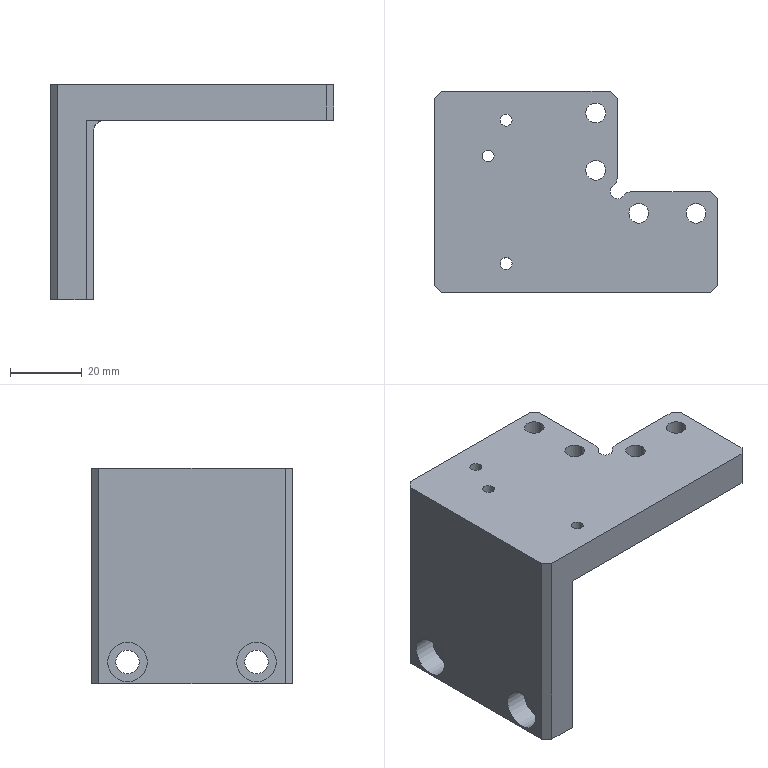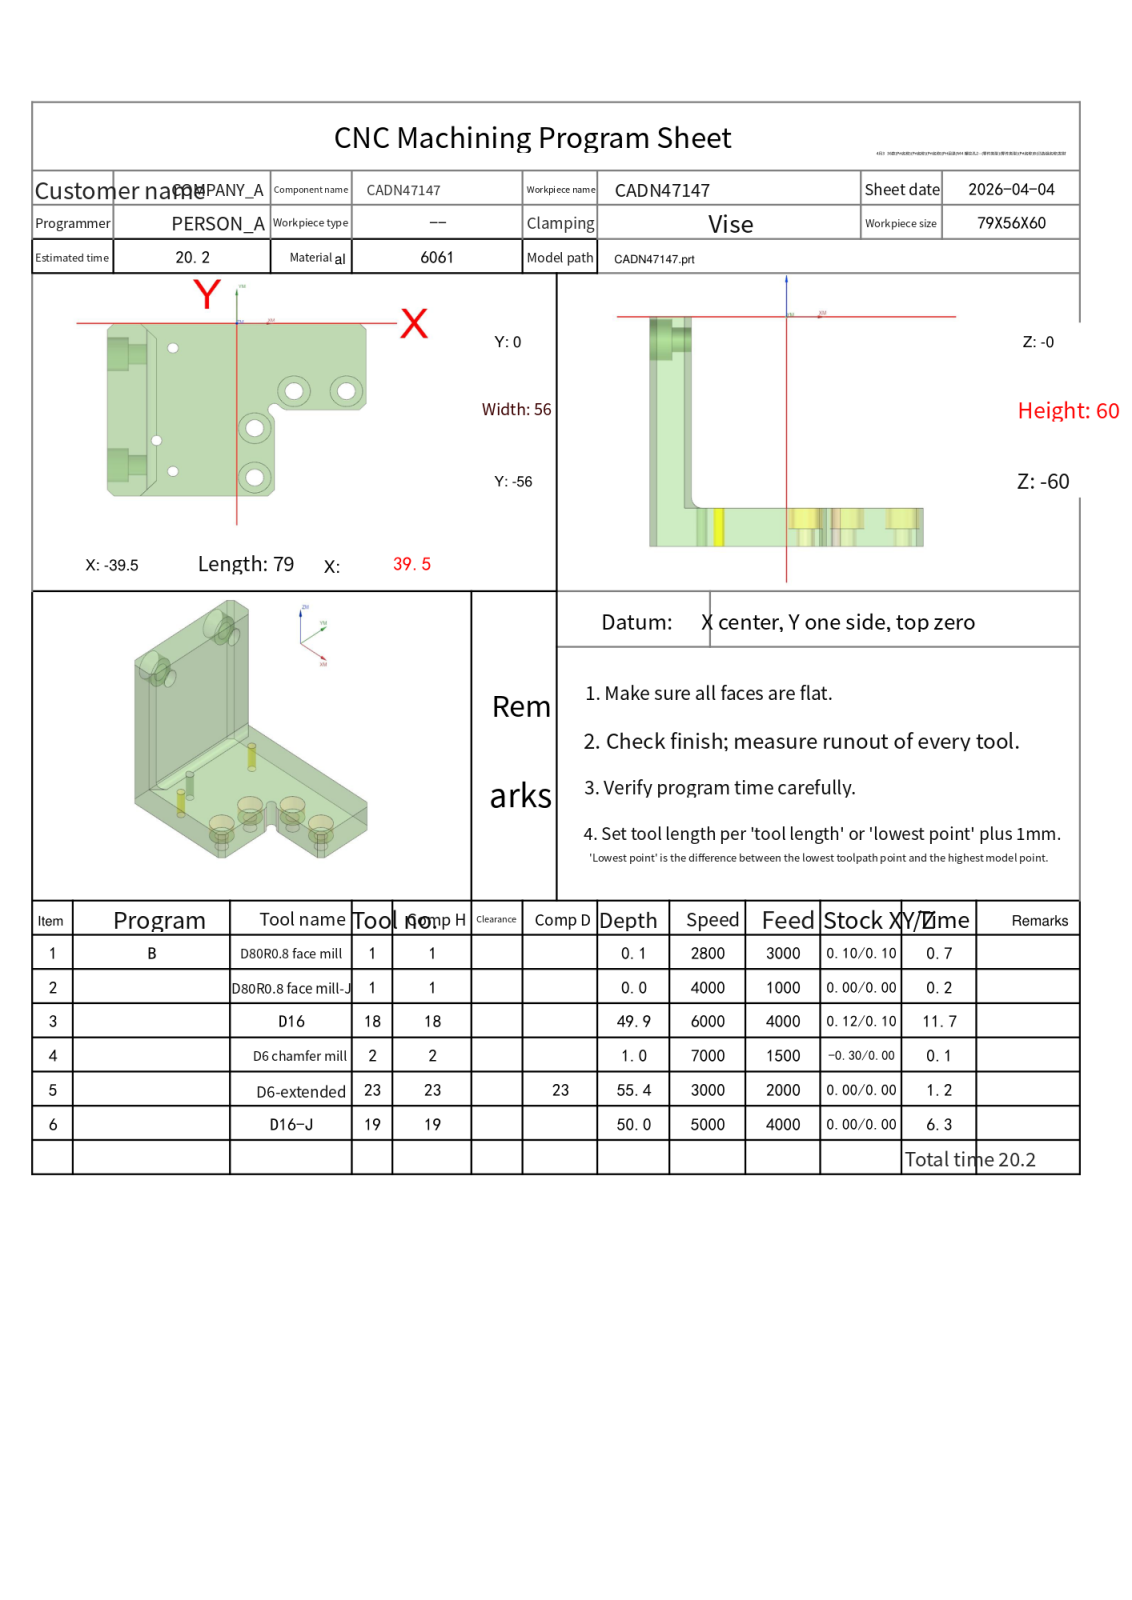NC program | NX | posted by the shop | part box 79 x 56 x 60 mm
Lines 11050 to 11358 of 15895:
N4 T02 M06
(D6 chamfer mill  D=6. R=0. H=02 ce=-0.30 di=0.00)
G00 G90 G54 X-26.8 Y-45.046 M03 S7000
G43 H02 Z20.
M08
Z2.5
G01 Y-53.953 Z-.742 F1500.
X-26.838 Y-54.16 Z-.819
X-26.919 Y-54.355 Z-.895
X-27.038 Y-54.528 Z-.972
X-27.093 Y-54.583 Z-1.
X-28.917 Y-56.407
G02 X-29.624 Y-56.7 I-.707 J.707
G01 X-37.376
G02 X-38.083 Y-56.407 I0.0 J1.
G01 X-39.907 Y-54.583
G02 X-40.2 Y-53.876 I.707 J.707
G01 Y-2.124
G02 X-39.907 Y-1.417 I1. J0.0
G01 X-38.083 Y.407
G02 X-37.376 Y.7 I.707 J-.707
G01 X-29.624
G02 X-28.917 Y.407 I0.0 J-1.
G01 X-27.093 Y-1.417
G02 X-26.8 Y-2.124 I-.707 J-.707
G01 Y-53.876
G02 X-27.093 Y-54.583 I-1. J0.0
G01 X-27.446 Y-54.936
Z1.5
G00 Z20.
G91 G28 Z0.0
M05
M09
G91 G28 Z0.0
M01
N5 T23 M06
(D6-extended  D=6. R=0. H=23 ce=0.10 di=0.00)
G00 G90 G54 X5.5 Y-34. M03 S3000
G43 H23 Z20.
M08
Z-49.7
G41 D23
G01 X5.493 Y-34.1 F2000.
G03 X6.444 Y-34.956 I.951 J.1
X7.4 Y-34. I0.0 J.956
X7.4 Y-34. Z-49.85 I-1.9 J0.0
X7.4 Y-34. Z-50. I-1.9 J0.0
X7.4 Y-34. Z-50.15 I-1.9 J0.0
X7.4 Y-34. Z-50.3 I-1.9 J0.0
X7.4 Y-34. Z-50.45 I-1.9 J0.0
X7.4 Y-34. Z-50.6 I-1.9 J0.0
X7.4 Y-34. Z-50.75 I-1.9 J0.0
X7.4 Y-34. Z-50.9 I-1.9 J0.0
X7.4 Y-34. Z-51.05 I-1.9 J0.0
X7.4 Y-34. Z-51.2 I-1.9 J0.0
X7.4 Y-34. Z-51.35 I-1.9 J0.0
X7.4 Y-34. Z-51.5 I-1.9 J0.0
X7.4 Y-34. Z-51.65 I-1.9 J0.0
X7.4 Y-34. Z-51.8 I-1.9 J0.0
X7.4 Y-34. Z-51.95 I-1.9 J0.0
X7.4 Y-34. Z-52.1 I-1.9 J0.0
X7.4 Y-34. Z-52.25 I-1.9 J0.0
X7.4 Y-34. Z-52.4 I-1.9 J0.0
X7.4 Y-34. Z-52.55 I-1.9 J0.0
X7.4 Y-34. Z-52.7 I-1.9 J0.0
X7.4 Y-34. Z-52.85 I-1.9 J0.0
X7.4 Y-34. Z-53. I-1.9 J0.0
X7.4 Y-34. Z-53.15 I-1.9 J0.0
X7.4 Y-34. Z-53.3 I-1.9 J0.0
X7.4 Y-34. Z-53.45 I-1.9 J0.0
X7.4 Y-34. Z-53.6 I-1.9 J0.0
X7.4 Y-34. Z-53.75 I-1.9 J0.0
X7.4 Y-34. Z-53.9 I-1.9 J0.0
X7.4 Y-34. Z-54.05 I-1.9 J0.0
X7.4 Y-34. Z-54.2 I-1.9 J0.0
X7.4 Y-34. Z-54.35 I-1.9 J0.0
X7.4 Y-34. Z-54.5 I-1.9 J0.0
X7.4 Y-34. Z-54.65 I-1.9 J0.0
X7.4 Y-34. Z-54.8 I-1.9 J0.0
X7.4 Y-34. Z-54.95 I-1.9 J0.0
X7.4 Y-34. Z-55.1 I-1.9 J0.0
X7.4 Y-34. Z-55.25 I-1.9 J0.0
X7.4 Y-34. Z-55.4 I-1.9 J0.0
X5.5 Y-32.1 I-1.9 J0.0
X3.6 Y-34. I0.0 J-1.9
X5.5 Y-35.9 I1.9 J0.0
X7.4 Y-34. I0.0 J1.9
X6.444 Y-33.044 I-.956 J0.0
X5.493 Y-33.9 I0.0 J-.956
G01 G40 X5.5 Y-34.
G00 Z20.
Y-50.
Z-49.7
G41 D23
G01 X5.493 Y-50.1
G03 X6.444 Y-50.956 I.951 J.1
X7.4 Y-50. I0.0 J.956
X7.4 Y-50. Z-49.85 I-1.9 J0.0
X7.4 Y-50. Z-50. I-1.9 J0.0
X7.4 Y-50. Z-50.15 I-1.9 J0.0
X7.4 Y-50. Z-50.3 I-1.9 J0.0
X7.4 Y-50. Z-50.45 I-1.9 J0.0
X7.4 Y-50. Z-50.6 I-1.9 J0.0
X7.4 Y-50. Z-50.75 I-1.9 J0.0
X7.4 Y-50. Z-50.9 I-1.9 J0.0
X7.4 Y-50. Z-51.05 I-1.9 J0.0
X7.4 Y-50. Z-51.2 I-1.9 J0.0
X7.4 Y-50. Z-51.35 I-1.9 J0.0
X7.4 Y-50. Z-51.5 I-1.9 J0.0
X7.4 Y-50. Z-51.65 I-1.9 J0.0
X7.4 Y-50. Z-51.8 I-1.9 J0.0
X7.4 Y-50. Z-51.95 I-1.9 J0.0
X7.4 Y-50. Z-52.1 I-1.9 J0.0
X7.4 Y-50. Z-52.25 I-1.9 J0.0
X7.4 Y-50. Z-52.4 I-1.9 J0.0
X7.4 Y-50. Z-52.55 I-1.9 J0.0
X7.4 Y-50. Z-52.7 I-1.9 J0.0
X7.4 Y-50. Z-52.85 I-1.9 J0.0
X7.4 Y-50. Z-53. I-1.9 J0.0
X7.4 Y-50. Z-53.15 I-1.9 J0.0
X7.4 Y-50. Z-53.3 I-1.9 J0.0
X7.4 Y-50. Z-53.45 I-1.9 J0.0
X7.4 Y-50. Z-53.6 I-1.9 J0.0
X7.4 Y-50. Z-53.75 I-1.9 J0.0
X7.4 Y-50. Z-53.9 I-1.9 J0.0
X7.4 Y-50. Z-54.05 I-1.9 J0.0
X7.4 Y-50. Z-54.2 I-1.9 J0.0
X7.4 Y-50. Z-54.35 I-1.9 J0.0
X7.4 Y-50. Z-54.5 I-1.9 J0.0
X7.4 Y-50. Z-54.65 I-1.9 J0.0
X7.4 Y-50. Z-54.8 I-1.9 J0.0
X7.4 Y-50. Z-54.95 I-1.9 J0.0
X7.4 Y-50. Z-55.1 I-1.9 J0.0
X7.4 Y-50. Z-55.25 I-1.9 J0.0
X7.4 Y-50. Z-55.4 I-1.9 J0.0
X5.5 Y-48.1 I-1.9 J0.0
X3.6 Y-50. I0.0 J-1.9
X5.5 Y-51.9 I1.9 J0.0
X7.4 Y-50. I0.0 J1.9
X6.444 Y-49.044 I-.956 J0.0
X5.493 Y-49.9 I0.0 J-.956
G01 G40 X5.5 Y-50.
G00 Z20.
X17.5 Y-22.
Z-49.7
G41 D23
G01 X17.493 Y-22.1
G03 X18.444 Y-22.956 I.951 J.1
X19.4 Y-22. I0.0 J.956
X19.4 Y-22. Z-49.85 I-1.9 J0.0
X19.4 Y-22. Z-50. I-1.9 J0.0
X19.4 Y-22. Z-50.15 I-1.9 J0.0
X19.4 Y-22. Z-50.3 I-1.9 J0.0
X19.4 Y-22. Z-50.45 I-1.9 J0.0
X19.4 Y-22. Z-50.6 I-1.9 J0.0
X19.4 Y-22. Z-50.75 I-1.9 J0.0
X19.4 Y-22. Z-50.9 I-1.9 J0.0
X19.4 Y-22. Z-51.05 I-1.9 J0.0
X19.4 Y-22. Z-51.2 I-1.9 J0.0
X19.4 Y-22. Z-51.35 I-1.9 J0.0
X19.4 Y-22. Z-51.5 I-1.9 J0.0
X19.4 Y-22. Z-51.65 I-1.9 J0.0
X19.4 Y-22. Z-51.8 I-1.9 J0.0
X19.4 Y-22. Z-51.95 I-1.9 J0.0
X19.4 Y-22. Z-52.1 I-1.9 J0.0
X19.4 Y-22. Z-52.25 I-1.9 J0.0
X19.4 Y-22. Z-52.4 I-1.9 J0.0
X19.4 Y-22. Z-52.55 I-1.9 J0.0
X19.4 Y-22. Z-52.7 I-1.9 J0.0
X19.4 Y-22. Z-52.85 I-1.9 J0.0
X19.4 Y-22. Z-53. I-1.9 J0.0
X19.4 Y-22. Z-53.15 I-1.9 J0.0
X19.4 Y-22. Z-53.3 I-1.9 J0.0
X19.4 Y-22. Z-53.45 I-1.9 J0.0
X19.4 Y-22. Z-53.6 I-1.9 J0.0
X19.4 Y-22. Z-53.75 I-1.9 J0.0
X19.4 Y-22. Z-53.9 I-1.9 J0.0
X19.4 Y-22. Z-54.05 I-1.9 J0.0
X19.4 Y-22. Z-54.2 I-1.9 J0.0
X19.4 Y-22. Z-54.35 I-1.9 J0.0
X19.4 Y-22. Z-54.5 I-1.9 J0.0
X19.4 Y-22. Z-54.65 I-1.9 J0.0
X19.4 Y-22. Z-54.8 I-1.9 J0.0
X19.4 Y-22. Z-54.95 I-1.9 J0.0
X19.4 Y-22. Z-55.1 I-1.9 J0.0
X19.4 Y-22. Z-55.25 I-1.9 J0.0
X19.4 Y-22. Z-55.4 I-1.9 J0.0
X17.5 Y-20.1 I-1.9 J0.0
X15.6 Y-22. I0.0 J-1.9
X17.5 Y-23.9 I1.9 J0.0
X19.4 Y-22. I0.0 J1.9
X18.444 Y-21.044 I-.956 J0.0
X17.493 Y-21.9 I0.0 J-.956
G01 G40 X17.5 Y-22.
G00 Z20.
X33.5
Z-49.7
G41 D23
G01 X33.493 Y-22.1
G03 X34.444 Y-22.956 I.951 J.1
X35.4 Y-22. I0.0 J.956
X35.4 Y-22. Z-49.85 I-1.9 J0.0
X35.4 Y-22. Z-50. I-1.9 J0.0
X35.4 Y-22. Z-50.15 I-1.9 J0.0
X35.4 Y-22. Z-50.3 I-1.9 J0.0
X35.4 Y-22. Z-50.45 I-1.9 J0.0
X35.4 Y-22. Z-50.6 I-1.9 J0.0
X35.4 Y-22. Z-50.75 I-1.9 J0.0
X35.4 Y-22. Z-50.9 I-1.9 J0.0
X35.4 Y-22. Z-51.05 I-1.9 J0.0
X35.4 Y-22. Z-51.2 I-1.9 J0.0
X35.4 Y-22. Z-51.35 I-1.9 J0.0
X35.4 Y-22. Z-51.5 I-1.9 J0.0
X35.4 Y-22. Z-51.65 I-1.9 J0.0
X35.4 Y-22. Z-51.8 I-1.9 J0.0
X35.4 Y-22. Z-51.95 I-1.9 J0.0
X35.4 Y-22. Z-52.1 I-1.9 J0.0
X35.4 Y-22. Z-52.25 I-1.9 J0.0
X35.4 Y-22. Z-52.4 I-1.9 J0.0
X35.4 Y-22. Z-52.55 I-1.9 J0.0
X35.4 Y-22. Z-52.7 I-1.9 J0.0
X35.4 Y-22. Z-52.85 I-1.9 J0.0
X35.4 Y-22. Z-53. I-1.9 J0.0
X35.4 Y-22. Z-53.15 I-1.9 J0.0
X35.4 Y-22. Z-53.3 I-1.9 J0.0
X35.4 Y-22. Z-53.45 I-1.9 J0.0
X35.4 Y-22. Z-53.6 I-1.9 J0.0
X35.4 Y-22. Z-53.75 I-1.9 J0.0
X35.4 Y-22. Z-53.9 I-1.9 J0.0
X35.4 Y-22. Z-54.05 I-1.9 J0.0
X35.4 Y-22. Z-54.2 I-1.9 J0.0
X35.4 Y-22. Z-54.35 I-1.9 J0.0
X35.4 Y-22. Z-54.5 I-1.9 J0.0
X35.4 Y-22. Z-54.65 I-1.9 J0.0
X35.4 Y-22. Z-54.8 I-1.9 J0.0
X35.4 Y-22. Z-54.95 I-1.9 J0.0
X35.4 Y-22. Z-55.1 I-1.9 J0.0
X35.4 Y-22. Z-55.25 I-1.9 J0.0
X35.4 Y-22. Z-55.4 I-1.9 J0.0
X33.5 Y-20.1 I-1.9 J0.0
X31.6 Y-22. I0.0 J-1.9
X33.5 Y-23.9 I1.9 J0.0
X35.4 Y-22. I0.0 J1.9
X34.444 Y-21.044 I-.956 J0.0
X33.493 Y-21.9 I0.0 J-.956
G01 G40 X33.5 Y-22.
G00 Z20.
G00 G90 X5.5 Y-34. M03 S3000
Z20.
Z-55.4
G01 X7.061 Y-34.351 F600.
X7.14 Y-34.36
G03 X7.5 Y-34. I0.0 J.36
X5.5 Y-32. I-2. J0.0
X3.5 Y-34. I0.0 J-2.
X5.5 Y-36. I2. J0.0
X7.5 Y-34. I0.0 J2.
X7.438 Y-33.505 I-2. J0.0
X7.089 Y-33.234 I-.349 J-.089
G01 X6.926 Y-33.274
X5.5 Y-34.
G00 Z20.
Y-50.
Z-55.4
G01 X7.061 Y-50.351
X7.14 Y-50.36
G03 X7.5 Y-50. I0.0 J.36
X5.5 Y-48. I-2. J0.0
X3.5 Y-50. I0.0 J-2.
X5.5 Y-52. I2. J0.0
X7.5 Y-50. I0.0 J2.
X7.438 Y-49.505 I-2. J0.0
X7.089 Y-49.234 I-.349 J-.089
G01 X6.926 Y-49.274
X5.5 Y-50.
G00 Z20.
X17.5 Y-22.
Z-55.4
G01 X19.061 Y-22.351
X19.14 Y-22.36
G03 X19.5 Y-22. I0.0 J.36
X17.5 Y-20. I-2. J0.0
X15.5 Y-22. I0.0 J-2.
X17.5 Y-24. I2. J0.0
X19.5 Y-22. I0.0 J2.
X19.438 Y-21.505 I-2. J0.0
X19.089 Y-21.234 I-.349 J-.089
G01 X18.926 Y-21.274
X17.5 Y-22.
G00 Z20.
X33.5
Z-55.4
G01 X35.061 Y-22.351
X35.14 Y-22.36
G03 X35.5 Y-22. I0.0 J.36
X33.5 Y-20. I-2. J0.0
X31.5 Y-22. I0.0 J-2.
X33.5 Y-24. I2. J0.0
X35.5 Y-22. I0.0 J2.
X35.438 Y-21.505 I-2. J0.0
X35.089 Y-21.234 I-.349 J-.089
G01 X34.926 Y-21.274
X33.5 Y-22.
G00 Z20.
G91 G28 Z0.0
M05
M09
G91 G28 Z0.0
M01